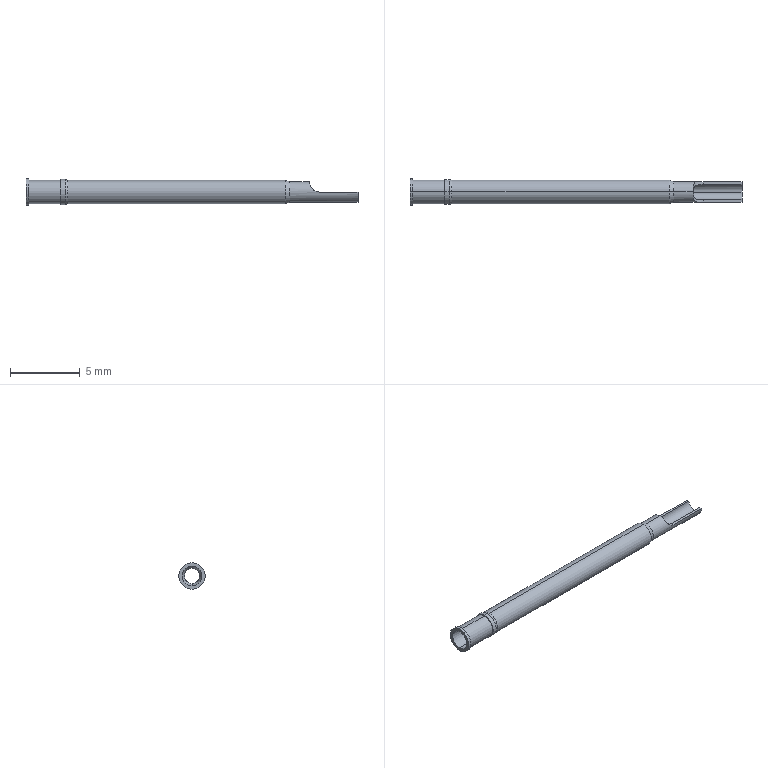Part | STEP file | Receptacle_NRB604 | 1 solid | 27 faces | box 23.8 x 1.9 x 1.9 mm | volume 15.467 mm3 | cylinder 15 | cone 6 | plane 6 | commonest cylinder face diameters 1.68 x4 1.47 x3 1.1 x2 1.4 x2 1.8 x2 1.9 x2
STEP:
#1=CARTESIAN_POINT('',(23.8,0.,-0.55));
#2=VERTEX_POINT('',#1);
#3=CARTESIAN_POINT('',(23.8,-0.55,0.));
#4=VERTEX_POINT('',#3);
#5=CARTESIAN_POINT('',(23.8,0.,0.));
#6=DIRECTION('',(-1.,0.,0.));
#7=DIRECTION('',(0.,0.,1.));
#8=AXIS2_PLACEMENT_3D('',#5,#6,#7);
#9=CIRCLE('',#8,0.55);
#10=EDGE_CURVE('',#2,#4,#9,.T.);
#11=ORIENTED_EDGE('',*,*,#10,.F.);
#12=CARTESIAN_POINT('',(18.901,0.,-0.55));
#13=VERTEX_POINT('',#12);
#14=CARTESIAN_POINT('',(23.8,0.,-0.55));
#15=DIRECTION('',(-1.,0.,0.));
#16=VECTOR('',#15,1000.);
#17=LINE('',#14,#16);
#18=EDGE_CURVE('',#2,#13,#17,.T.);
#19=ORIENTED_EDGE('',*,*,#18,.T.);
#20=CARTESIAN_POINT('',(18.901,0.,0.55));
#21=VERTEX_POINT('',#20);
#22=CARTESIAN_POINT('',(18.901,0.,0.));
#23=DIRECTION('',(-1.,0.,0.));
#24=DIRECTION('',(0.,0.,1.));
#25=AXIS2_PLACEMENT_3D('',#22,#23,#24);
#26=CIRCLE('',#25,0.55);
#27=EDGE_CURVE('',#13,#21,#26,.T.);
#28=ORIENTED_EDGE('',*,*,#27,.T.);
#29=CARTESIAN_POINT('',(20.324,0.,0.55));
#30=VERTEX_POINT('',#29);
#31=CARTESIAN_POINT('',(23.8,0.,0.55));
#32=DIRECTION('',(-1.,0.,0.));
#33=VECTOR('',#32,1000.);
#34=LINE('',#31,#33);
#35=EDGE_CURVE('',#30,#21,#34,.T.);
#36=ORIENTED_EDGE('',*,*,#35,.F.);
#37=CARTESIAN_POINT('',(21.035,-0.55,0.));
#38=VERTEX_POINT('',#37);
#39=CARTESIAN_POINT('',(21.035,-0.55,0.));
#40=CARTESIAN_POINT('',(20.928,-0.55,0.));
#41=CARTESIAN_POINT('',(20.825,-0.5513,0.02284));
#42=CARTESIAN_POINT('',(20.681,-0.5432,0.08883));
#43=CARTESIAN_POINT('',(20.636,-0.5387,0.1156));
#44=CARTESIAN_POINT('',(20.553,-0.5214,0.1779));
#45=CARTESIAN_POINT('',(20.515,-0.5085,0.2137));
#46=CARTESIAN_POINT('',(20.417,-0.4516,0.3248));
#47=CARTESIAN_POINT('',(20.375,-0.3857,0.4055));
#48=CARTESIAN_POINT('',(20.33,-0.2125,0.5177));
#49=CARTESIAN_POINT('',(20.324,-0.1056,0.55));
#50=CARTESIAN_POINT('',(20.324,0.,0.55));
#51=B_SPLINE_CURVE_WITH_KNOTS('',3,(#39,#40,#41,#42,#43,#44,#45,#46,#47,#48,#49,#50),.UNSPECIFIED.,.F.,.F.,(4,2,2,2,2,4),(0.,0.0003137,0.0004705,0.0006274,0.0009411,0.001255),.UNSPECIFIED.);
#52=EDGE_CURVE('',#38,#30,#51,.T.);
#53=ORIENTED_EDGE('',*,*,#52,.F.);
#54=CARTESIAN_POINT('',(23.8,-0.55,0.));
#55=DIRECTION('',(-1.,0.,0.));
#56=VECTOR('',#55,1000.);
#57=LINE('',#54,#56);
#58=EDGE_CURVE('',#4,#38,#57,.T.);
#59=ORIENTED_EDGE('',*,*,#58,.F.);
#60=EDGE_LOOP('',(#11,#19,#28,#36,#53,#59));
#61=FACE_OUTER_BOUND('',#60,.T.);
#62=CARTESIAN_POINT('',(23.8,0.,0.));
#63=DIRECTION('',(-1.,0.,0.));
#64=DIRECTION('',(0.,0.,1.));
#65=AXIS2_PLACEMENT_3D('',#62,#63,#64);
#66=CYLINDRICAL_SURFACE('',#65,0.55);
#67=ADVANCED_FACE('',(#61),#66,.F.);
#68=ORIENTED_EDGE('',*,*,#27,.F.);
#69=CARTESIAN_POINT('',(18.6,0.,-0.7));
#70=VERTEX_POINT('',#69);
#71=CARTESIAN_POINT('',(18.901,0.,-0.55));
#72=DIRECTION('',(-0.8949,0.,-0.4462));
#73=VECTOR('',#72,1000.);
#74=LINE('',#71,#73);
#75=EDGE_CURVE('',#13,#70,#74,.T.);
#76=ORIENTED_EDGE('',*,*,#75,.T.);
#77=CARTESIAN_POINT('',(18.6,0.,0.7));
#78=VERTEX_POINT('',#77);
#79=CARTESIAN_POINT('',(18.6,0.,0.));
#80=DIRECTION('',(-1.,0.,0.));
#81=DIRECTION('',(0.,0.,1.));
#82=AXIS2_PLACEMENT_3D('',#79,#80,#81);
#83=CIRCLE('',#82,0.7);
#84=EDGE_CURVE('',#70,#78,#83,.T.);
#85=ORIENTED_EDGE('',*,*,#84,.T.);
#86=CARTESIAN_POINT('',(18.901,0.,0.55));
#87=DIRECTION('',(-0.8949,0.,0.4462));
#88=VECTOR('',#87,1000.);
#89=LINE('',#86,#88);
#90=EDGE_CURVE('',#21,#78,#89,.T.);
#91=ORIENTED_EDGE('',*,*,#90,.F.);
#92=EDGE_LOOP('',(#68,#76,#85,#91));
#93=FACE_OUTER_BOUND('',#92,.T.);
#94=CARTESIAN_POINT('',(18.901,0.,0.));
#95=DIRECTION('',(-1.,0.,0.));
#96=DIRECTION('',(0.,0.,1.));
#97=AXIS2_PLACEMENT_3D('',#94,#95,#96);
#98=CONICAL_SURFACE('',#97,0.55,0.4625);
#99=ADVANCED_FACE('',(#93),#98,.F.);
#100=ORIENTED_EDGE('',*,*,#84,.F.);
#101=CARTESIAN_POINT('',(0.,0.,-0.7));
#102=VERTEX_POINT('',#101);
#103=CARTESIAN_POINT('',(23.8,0.,-0.7));
#104=DIRECTION('',(-1.,0.,0.));
#105=VECTOR('',#104,1000.);
#106=LINE('',#103,#105);
#107=EDGE_CURVE('',#70,#102,#106,.T.);
#108=ORIENTED_EDGE('',*,*,#107,.T.);
#109=CARTESIAN_POINT('',(0.,0.,0.7));
#110=VERTEX_POINT('',#109);
#111=CARTESIAN_POINT('',(0.,0.,0.));
#112=DIRECTION('',(-1.,0.,0.));
#113=DIRECTION('',(0.,0.,1.));
#114=AXIS2_PLACEMENT_3D('',#111,#112,#113);
#115=CIRCLE('',#114,0.7);
#116=EDGE_CURVE('',#102,#110,#115,.T.);
#117=ORIENTED_EDGE('',*,*,#116,.T.);
#118=CARTESIAN_POINT('',(23.8,0.,0.7));
#119=DIRECTION('',(-1.,0.,0.));
#120=VECTOR('',#119,1000.);
#121=LINE('',#118,#120);
#122=EDGE_CURVE('',#78,#110,#121,.T.);
#123=ORIENTED_EDGE('',*,*,#122,.F.);
#124=EDGE_LOOP('',(#100,#108,#117,#123));
#125=FACE_OUTER_BOUND('',#124,.T.);
#126=CARTESIAN_POINT('',(23.8,0.,0.));
#127=DIRECTION('',(-1.,0.,0.));
#128=DIRECTION('',(0.,0.,1.));
#129=AXIS2_PLACEMENT_3D('',#126,#127,#128);
#130=CYLINDRICAL_SURFACE('',#129,0.7);
#131=ADVANCED_FACE('',(#125),#130,.F.);
#132=CARTESIAN_POINT('',(23.8,0.735,0.));
#133=VERTEX_POINT('',#132);
#134=CARTESIAN_POINT('',(23.8,0.,-0.735));
#135=VERTEX_POINT('',#134);
#136=CARTESIAN_POINT('',(23.8,0.,0.));
#137=DIRECTION('',(-1.,0.,0.));
#138=DIRECTION('',(0.,0.,1.));
#139=AXIS2_PLACEMENT_3D('',#136,#137,#138);
#140=CIRCLE('',#139,0.735);
#141=EDGE_CURVE('',#133,#135,#140,.T.);
#142=ORIENTED_EDGE('',*,*,#141,.T.);
#143=CARTESIAN_POINT('',(18.9,0.,-0.735));
#144=VERTEX_POINT('',#143);
#145=CARTESIAN_POINT('',(23.8,0.,-0.735));
#146=DIRECTION('',(-1.,0.,0.));
#147=VECTOR('',#146,1000.);
#148=LINE('',#145,#147);
#149=EDGE_CURVE('',#135,#144,#148,.T.);
#150=ORIENTED_EDGE('',*,*,#149,.T.);
#151=CARTESIAN_POINT('',(18.9,0.,0.735));
#152=VERTEX_POINT('',#151);
#153=CARTESIAN_POINT('',(18.9,0.,0.));
#154=DIRECTION('',(-1.,0.,0.));
#155=DIRECTION('',(0.,0.,1.));
#156=AXIS2_PLACEMENT_3D('',#153,#154,#155);
#157=CIRCLE('',#156,0.735);
#158=EDGE_CURVE('',#152,#144,#157,.T.);
#159=ORIENTED_EDGE('',*,*,#158,.F.);
#160=CARTESIAN_POINT('',(20.3,0.,0.735));
#161=VERTEX_POINT('',#160);
#162=CARTESIAN_POINT('',(23.8,0.,0.735));
#163=DIRECTION('',(-1.,0.,0.));
#164=VECTOR('',#163,1000.);
#165=LINE('',#162,#164);
#166=EDGE_CURVE('',#161,#152,#165,.T.);
#167=ORIENTED_EDGE('',*,*,#166,.F.);
#168=CARTESIAN_POINT('',(21.035,0.735,0.));
#169=VERTEX_POINT('',#168);
#170=CARTESIAN_POINT('',(20.3,0.,0.735));
#171=CARTESIAN_POINT('',(20.3,0.1314,0.735));
#172=CARTESIAN_POINT('',(20.298,0.2613,0.6991));
#173=CARTESIAN_POINT('',(20.316,0.4842,0.5679));
#174=CARTESIAN_POINT('',(20.34,0.5775,0.4695));
#175=CARTESIAN_POINT('',(20.456,0.6946,0.2672));
#176=CARTESIAN_POINT('',(20.549,0.7186,0.1684));
#177=CARTESIAN_POINT('',(20.774,0.7372,0.03573));
#178=CARTESIAN_POINT('',(20.903,0.735,0.));
#179=CARTESIAN_POINT('',(21.035,0.735,0.));
#180=B_SPLINE_CURVE_WITH_KNOTS('',3,(#170,#171,#172,#173,#174,#175,#176,#177,#178,#179),.UNSPECIFIED.,.F.,.F.,(4,2,2,2,4),(0.001558,0.001947,0.002336,0.002725,0.003114),.UNSPECIFIED.);
#181=EDGE_CURVE('',#161,#169,#180,.T.);
#182=ORIENTED_EDGE('',*,*,#181,.T.);
#183=CARTESIAN_POINT('',(23.8,0.735,0.));
#184=DIRECTION('',(-1.,0.,0.));
#185=VECTOR('',#184,1000.);
#186=LINE('',#183,#185);
#187=EDGE_CURVE('',#133,#169,#186,.T.);
#188=ORIENTED_EDGE('',*,*,#187,.F.);
#189=EDGE_LOOP('',(#142,#150,#159,#167,#182,#188));
#190=FACE_OUTER_BOUND('',#189,.T.);
#191=CARTESIAN_POINT('',(23.8,0.,0.));
#192=DIRECTION('',(-1.,0.,0.));
#193=DIRECTION('',(0.,0.,1.));
#194=AXIS2_PLACEMENT_3D('',#191,#192,#193);
#195=CYLINDRICAL_SURFACE('',#194,0.735);
#196=ADVANCED_FACE('',(#190),#195,.T.);
#197=ORIENTED_EDGE('',*,*,#158,.T.);
#198=CARTESIAN_POINT('',(18.6,0.,-0.84));
#199=VERTEX_POINT('',#198);
#200=CARTESIAN_POINT('',(18.9,0.,-0.735));
#201=DIRECTION('',(-0.9439,0.,-0.3304));
#202=VECTOR('',#201,1000.);
#203=LINE('',#200,#202);
#204=EDGE_CURVE('',#144,#199,#203,.T.);
#205=ORIENTED_EDGE('',*,*,#204,.T.);
#206=CARTESIAN_POINT('',(18.6,0.,0.84));
#207=VERTEX_POINT('',#206);
#208=CARTESIAN_POINT('',(18.6,0.,0.));
#209=DIRECTION('',(-1.,0.,0.));
#210=DIRECTION('',(0.,0.,1.));
#211=AXIS2_PLACEMENT_3D('',#208,#209,#210);
#212=CIRCLE('',#211,0.84);
#213=EDGE_CURVE('',#207,#199,#212,.T.);
#214=ORIENTED_EDGE('',*,*,#213,.F.);
#215=CARTESIAN_POINT('',(18.9,0.,0.735));
#216=DIRECTION('',(-0.9439,0.,0.3304));
#217=VECTOR('',#216,1000.);
#218=LINE('',#215,#217);
#219=EDGE_CURVE('',#152,#207,#218,.T.);
#220=ORIENTED_EDGE('',*,*,#219,.F.);
#221=EDGE_LOOP('',(#197,#205,#214,#220));
#222=FACE_OUTER_BOUND('',#221,.T.);
#223=CARTESIAN_POINT('',(18.9,0.,0.));
#224=DIRECTION('',(-1.,0.,0.));
#225=DIRECTION('',(0.,0.,1.));
#226=AXIS2_PLACEMENT_3D('',#223,#224,#225);
#227=CONICAL_SURFACE('',#226,0.735,0.3367);
#228=ADVANCED_FACE('',(#222),#227,.T.);
#229=ORIENTED_EDGE('',*,*,#213,.T.);
#230=CARTESIAN_POINT('',(3.,0.,-0.84));
#231=VERTEX_POINT('',#230);
#232=CARTESIAN_POINT('',(23.8,0.,-0.84));
#233=DIRECTION('',(-1.,0.,0.));
#234=VECTOR('',#233,1000.);
#235=LINE('',#232,#234);
#236=EDGE_CURVE('',#199,#231,#235,.T.);
#237=ORIENTED_EDGE('',*,*,#236,.T.);
#238=CARTESIAN_POINT('',(3.,0.,0.84));
#239=VERTEX_POINT('',#238);
#240=CARTESIAN_POINT('',(3.,0.,0.));
#241=DIRECTION('',(-1.,0.,0.));
#242=DIRECTION('',(0.,0.,1.));
#243=AXIS2_PLACEMENT_3D('',#240,#241,#242);
#244=CIRCLE('',#243,0.84);
#245=EDGE_CURVE('',#239,#231,#244,.T.);
#246=ORIENTED_EDGE('',*,*,#245,.F.);
#247=CARTESIAN_POINT('',(23.8,0.,0.84));
#248=DIRECTION('',(-1.,0.,0.));
#249=VECTOR('',#248,1000.);
#250=LINE('',#247,#249);
#251=EDGE_CURVE('',#207,#239,#250,.T.);
#252=ORIENTED_EDGE('',*,*,#251,.F.);
#253=EDGE_LOOP('',(#229,#237,#246,#252));
#254=FACE_OUTER_BOUND('',#253,.T.);
#255=CARTESIAN_POINT('',(23.8,0.,0.));
#256=DIRECTION('',(-1.,0.,0.));
#257=DIRECTION('',(0.,0.,1.));
#258=AXIS2_PLACEMENT_3D('',#255,#256,#257);
#259=CYLINDRICAL_SURFACE('',#258,0.84);
#260=ADVANCED_FACE('',(#254),#259,.T.);
#261=ORIENTED_EDGE('',*,*,#245,.T.);
#262=CARTESIAN_POINT('',(2.8,0.,-0.9));
#263=VERTEX_POINT('',#262);
#264=CARTESIAN_POINT('',(3.,0.,-0.84));
#265=DIRECTION('',(-0.9578,0.,-0.2873));
#266=VECTOR('',#265,1000.);
#267=LINE('',#264,#266);
#268=EDGE_CURVE('',#231,#263,#267,.T.);
#269=ORIENTED_EDGE('',*,*,#268,.T.);
#270=CARTESIAN_POINT('',(2.8,0.,0.9));
#271=VERTEX_POINT('',#270);
#272=CARTESIAN_POINT('',(2.8,0.,0.));
#273=DIRECTION('',(-1.,0.,0.));
#274=DIRECTION('',(0.,0.,1.));
#275=AXIS2_PLACEMENT_3D('',#272,#273,#274);
#276=CIRCLE('',#275,0.9);
#277=EDGE_CURVE('',#271,#263,#276,.T.);
#278=ORIENTED_EDGE('',*,*,#277,.F.);
#279=CARTESIAN_POINT('',(3.,0.,0.84));
#280=DIRECTION('',(-0.9578,0.,0.2873));
#281=VECTOR('',#280,1000.);
#282=LINE('',#279,#281);
#283=EDGE_CURVE('',#239,#271,#282,.T.);
#284=ORIENTED_EDGE('',*,*,#283,.F.);
#285=EDGE_LOOP('',(#261,#269,#278,#284));
#286=FACE_OUTER_BOUND('',#285,.T.);
#287=CARTESIAN_POINT('',(3.,0.,0.));
#288=DIRECTION('',(-1.,0.,0.));
#289=DIRECTION('',(0.,0.,1.));
#290=AXIS2_PLACEMENT_3D('',#287,#288,#289);
#291=CONICAL_SURFACE('',#290,0.84,0.2915);
#292=ADVANCED_FACE('',(#286),#291,.T.);
#293=ORIENTED_EDGE('',*,*,#277,.T.);
#294=CARTESIAN_POINT('',(2.5,0.,-0.9));
#295=VERTEX_POINT('',#294);
#296=CARTESIAN_POINT('',(23.8,0.,-0.9));
#297=DIRECTION('',(-1.,0.,0.));
#298=VECTOR('',#297,1000.);
#299=LINE('',#296,#298);
#300=EDGE_CURVE('',#263,#295,#299,.T.);
#301=ORIENTED_EDGE('',*,*,#300,.T.);
#302=CARTESIAN_POINT('',(2.5,0.,0.9));
#303=VERTEX_POINT('',#302);
#304=CARTESIAN_POINT('',(2.5,0.,0.));
#305=DIRECTION('',(-1.,0.,0.));
#306=DIRECTION('',(0.,0.,1.));
#307=AXIS2_PLACEMENT_3D('',#304,#305,#306);
#308=CIRCLE('',#307,0.9);
#309=EDGE_CURVE('',#303,#295,#308,.T.);
#310=ORIENTED_EDGE('',*,*,#309,.F.);
#311=CARTESIAN_POINT('',(23.8,0.,0.9));
#312=DIRECTION('',(-1.,0.,0.));
#313=VECTOR('',#312,1000.);
#314=LINE('',#311,#313);
#315=EDGE_CURVE('',#271,#303,#314,.T.);
#316=ORIENTED_EDGE('',*,*,#315,.F.);
#317=EDGE_LOOP('',(#293,#301,#310,#316));
#318=FACE_OUTER_BOUND('',#317,.T.);
#319=CARTESIAN_POINT('',(23.8,0.,0.));
#320=DIRECTION('',(-1.,0.,0.));
#321=DIRECTION('',(0.,0.,1.));
#322=AXIS2_PLACEMENT_3D('',#319,#320,#321);
#323=CYLINDRICAL_SURFACE('',#322,0.9);
#324=ADVANCED_FACE('',(#318),#323,.T.);
#325=CARTESIAN_POINT('',(2.5,0.,0.84));
#326=VERTEX_POINT('',#325);
#327=CARTESIAN_POINT('',(2.5,0.,-0.84));
#328=VERTEX_POINT('',#327);
#329=CARTESIAN_POINT('',(2.5,0.,0.));
#330=DIRECTION('',(-1.,0.,0.));
#331=DIRECTION('',(0.,0.,1.));
#332=AXIS2_PLACEMENT_3D('',#329,#330,#331);
#333=CIRCLE('',#332,0.84);
#334=EDGE_CURVE('',#326,#328,#333,.T.);
#335=ORIENTED_EDGE('',*,*,#334,.T.);
#336=CARTESIAN_POINT('',(0.2,0.,-0.84));
#337=VERTEX_POINT('',#336);
#338=CARTESIAN_POINT('',(23.8,0.,-0.84));
#339=DIRECTION('',(-1.,0.,0.));
#340=VECTOR('',#339,1000.);
#341=LINE('',#338,#340);
#342=EDGE_CURVE('',#328,#337,#341,.T.);
#343=ORIENTED_EDGE('',*,*,#342,.T.);
#344=CARTESIAN_POINT('',(0.2,0.,0.84));
#345=VERTEX_POINT('',#344);
#346=CARTESIAN_POINT('',(0.2,0.,0.));
#347=DIRECTION('',(-1.,0.,0.));
#348=DIRECTION('',(0.,0.,1.));
#349=AXIS2_PLACEMENT_3D('',#346,#347,#348);
#350=CIRCLE('',#349,0.84);
#351=EDGE_CURVE('',#345,#337,#350,.T.);
#352=ORIENTED_EDGE('',*,*,#351,.F.);
#353=CARTESIAN_POINT('',(23.8,0.,0.84));
#354=DIRECTION('',(-1.,0.,0.));
#355=VECTOR('',#354,1000.);
#356=LINE('',#353,#355);
#357=EDGE_CURVE('',#326,#345,#356,.T.);
#358=ORIENTED_EDGE('',*,*,#357,.F.);
#359=EDGE_LOOP('',(#335,#343,#352,#358));
#360=FACE_OUTER_BOUND('',#359,.T.);
#361=CARTESIAN_POINT('',(23.8,0.,0.));
#362=DIRECTION('',(-1.,0.,0.));
#363=DIRECTION('',(0.,0.,1.));
#364=AXIS2_PLACEMENT_3D('',#361,#362,#363);
#365=CYLINDRICAL_SURFACE('',#364,0.84);
#366=ADVANCED_FACE('',(#360),#365,.T.);
#367=CARTESIAN_POINT('',(0.2,0.,0.95));
#368=VERTEX_POINT('',#367);
#369=CARTESIAN_POINT('',(0.2,0.,-0.95));
#370=VERTEX_POINT('',#369);
#371=CARTESIAN_POINT('',(0.2,0.,0.));
#372=DIRECTION('',(-1.,0.,0.));
#373=DIRECTION('',(0.,0.,1.));
#374=AXIS2_PLACEMENT_3D('',#371,#372,#373);
#375=CIRCLE('',#374,0.95);
#376=EDGE_CURVE('',#368,#370,#375,.T.);
#377=ORIENTED_EDGE('',*,*,#376,.T.);
#378=CARTESIAN_POINT('',(0.,0.,-0.95));
#379=VERTEX_POINT('',#378);
#380=CARTESIAN_POINT('',(23.8,0.,-0.95));
#381=DIRECTION('',(-1.,0.,0.));
#382=VECTOR('',#381,1000.);
#383=LINE('',#380,#382);
#384=EDGE_CURVE('',#370,#379,#383,.T.);
#385=ORIENTED_EDGE('',*,*,#384,.T.);
#386=CARTESIAN_POINT('',(0.,0.,0.95));
#387=VERTEX_POINT('',#386);
#388=CARTESIAN_POINT('',(0.,0.,0.));
#389=DIRECTION('',(-1.,0.,0.));
#390=DIRECTION('',(0.,0.,1.));
#391=AXIS2_PLACEMENT_3D('',#388,#389,#390);
#392=CIRCLE('',#391,0.95);
#393=EDGE_CURVE('',#387,#379,#392,.T.);
#394=ORIENTED_EDGE('',*,*,#393,.F.);
#395=CARTESIAN_POINT('',(23.8,0.,0.95));
#396=DIRECTION('',(-1.,0.,0.));
#397=VECTOR('',#396,1000.);
#398=LINE('',#395,#397);
#399=EDGE_CURVE('',#368,#387,#398,.T.);
#400=ORIENTED_EDGE('',*,*,#399,.F.);
#401=EDGE_LOOP('',(#377,#385,#394,#400));
#402=FACE_OUTER_BOUND('',#401,.T.);
#403=CARTESIAN_POINT('',(23.8,0.,0.));
#404=DIRECTION('',(-1.,0.,0.));
#405=DIRECTION('',(0.,0.,1.));
#406=AXIS2_PLACEMENT_3D('',#403,#404,#405);
#407=CYLINDRICAL_SURFACE('',#406,0.95);
#408=ADVANCED_FACE('',(#402),#407,.T.);
#409=ORIENTED_EDGE('',*,*,#393,.T.);
#410=CARTESIAN_POINT('',(0.,0.,0.));
#411=DIRECTION('',(-1.,0.,0.));
#412=DIRECTION('',(0.,0.,1.));
#413=AXIS2_PLACEMENT_3D('',#410,#411,#412);
#414=CIRCLE('',#413,0.95);
#415=EDGE_CURVE('',#379,#387,#414,.T.);
#416=ORIENTED_EDGE('',*,*,#415,.T.);
#417=EDGE_LOOP('',(#409,#416));
#418=FACE_OUTER_BOUND('',#417,.T.);
#419=CARTESIAN_POINT('',(0.,0.,0.));
#420=DIRECTION('',(-1.,0.,0.));
#421=DIRECTION('',(0.,0.,1.));
#422=AXIS2_PLACEMENT_3D('',#419,#420,#421);
#423=CIRCLE('',#422,0.7);
#424=EDGE_CURVE('',#110,#102,#423,.T.);
#425=ORIENTED_EDGE('',*,*,#424,.F.);
#426=ORIENTED_EDGE('',*,*,#116,.F.);
#427=EDGE_LOOP('',(#425,#426));
#428=FACE_BOUND('',#427,.T.);
#429=CARTESIAN_POINT('',(0.,0.,0.));
#430=DIRECTION('',(1.,0.,0.));
#431=DIRECTION('',(0.,0.,-1.));
#432=AXIS2_PLACEMENT_3D('',#429,#430,#431);
#433=PLANE('',#432);
#434=ADVANCED_FACE('',(#418,#428),#433,.F.);
#435=ORIENTED_EDGE('',*,*,#141,.F.);
#436=CARTESIAN_POINT('',(23.8,0.55,0.));
#437=VERTEX_POINT('',#436);
#438=CARTESIAN_POINT('',(23.8,-0.735,0.));
#439=DIRECTION('',(0.,1.,0.));
#440=VECTOR('',#439,1000.);
#441=LINE('',#438,#440);
#442=EDGE_CURVE('',#437,#133,#441,.T.);
#443=ORIENTED_EDGE('',*,*,#442,.F.);
#444=CARTESIAN_POINT('',(23.8,0.,0.));
#445=DIRECTION('',(-1.,0.,0.));
#446=DIRECTION('',(0.,0.,1.));
#447=AXIS2_PLACEMENT_3D('',#444,#445,#446);
#448=CIRCLE('',#447,0.55);
#449=EDGE_CURVE('',#437,#2,#448,.T.);
#450=ORIENTED_EDGE('',*,*,#449,.T.);
#451=ORIENTED_EDGE('',*,*,#10,.T.);
#452=CARTESIAN_POINT('',(23.8,-0.735,0.));
#453=VERTEX_POINT('',#452);
#454=CARTESIAN_POINT('',(23.8,-0.735,0.));
#455=DIRECTION('',(0.,1.,0.));
#456=VECTOR('',#455,1000.);
#457=LINE('',#454,#456);
#458=EDGE_CURVE('',#453,#4,#457,.T.);
#459=ORIENTED_EDGE('',*,*,#458,.F.);
#460=CARTESIAN_POINT('',(23.8,0.,0.));
#461=DIRECTION('',(-1.,0.,0.));
#462=DIRECTION('',(0.,0.,1.));
#463=AXIS2_PLACEMENT_3D('',#460,#461,#462);
#464=CIRCLE('',#463,0.735);
#465=EDGE_CURVE('',#135,#453,#464,.T.);
#466=ORIENTED_EDGE('',*,*,#465,.F.);
#467=EDGE_LOOP('',(#435,#443,#450,#451,#459,#466));
#468=FACE_OUTER_BOUND('',#467,.T.);
#469=CARTESIAN_POINT('',(23.8,0.735,0.));
#470=DIRECTION('',(-1.,0.,0.));
#471=DIRECTION('',(0.,0.,1.));
#472=AXIS2_PLACEMENT_3D('',#469,#470,#471);
#473=PLANE('',#472);
#474=ADVANCED_FACE('',(#468),#473,.F.);
#475=ORIENTED_EDGE('',*,*,#384,.F.);
#476=CARTESIAN_POINT('',(0.2,0.,0.));
#477=DIRECTION('',(-1.,0.,0.));
#478=DIRECTION('',(0.,0.,1.));
#479=AXIS2_PLACEMENT_3D('',#476,#477,#478);
#480=CIRCLE('',#479,0.95);
#481=EDGE_CURVE('',#370,#368,#480,.T.);
#482=ORIENTED_EDGE('',*,*,#481,.T.);
#483=ORIENTED_EDGE('',*,*,#399,.T.);
#484=ORIENTED_EDGE('',*,*,#415,.F.);
#485=EDGE_LOOP('',(#475,#482,#483,#484));
#486=FACE_OUTER_BOUND('',#485,.T.);
#487=CARTESIAN_POINT('',(23.8,0.,0.));
#488=DIRECTION('',(-1.,0.,0.));
#489=DIRECTION('',(0.,0.,1.));
#490=AXIS2_PLACEMENT_3D('',#487,#488,#489);
#491=CYLINDRICAL_SURFACE('',#490,0.95);
#492=ADVANCED_FACE('',(#486),#491,.T.);
#493=ORIENTED_EDGE('',*,*,#376,.F.);
#494=ORIENTED_EDGE('',*,*,#481,.F.);
#495=EDGE_LOOP('',(#493,#494));
#496=FACE_OUTER_BOUND('',#495,.T.);
#497=ORIENTED_EDGE('',*,*,#351,.T.);
#498=CARTESIAN_POINT('',(0.2,0.,0.));
#499=DIRECTION('',(-1.,0.,0.));
#500=DIRECTION('',(0.,0.,1.));
#501=AXIS2_PLACEMENT_3D('',#498,#499,#500);
#502=CIRCLE('',#501,0.84);
#503=EDGE_CURVE('',#337,#345,#502,.T.);
#504=ORIENTED_EDGE('',*,*,#503,.T.);
#505=EDGE_LOOP('',(#497,#504));
#506=FACE_BOUND('',#505,.T.);
#507=CARTESIAN_POINT('',(0.2,0.95,0.));
#508=DIRECTION('',(-1.,0.,0.));
#509=DIRECTION('',(0.,0.,1.));
#510=AXIS2_PLACEMENT_3D('',#507,#508,#509);
#511=PLANE('',#510);
#512=ADVANCED_FACE('',(#496,#506),#511,.F.);
#513=ORIENTED_EDGE('',*,*,#342,.F.);
#514=CARTESIAN_POINT('',(2.5,0.,0.));
#515=DIRECTION('',(-1.,0.,0.));
#516=DIRECTION('',(0.,0.,1.));
#517=AXIS2_PLACEMENT_3D('',#514,#515,#516);
#518=CIRCLE('',#517,0.84);
#519=EDGE_CURVE('',#328,#326,#518,.T.);
#520=ORIENTED_EDGE('',*,*,#519,.T.);
#521=ORIENTED_EDGE('',*,*,#357,.T.);
#522=ORIENTED_EDGE('',*,*,#503,.F.);
#523=EDGE_LOOP('',(#513,#520,#521,#522));
#524=FACE_OUTER_BOUND('',#523,.T.);
#525=CARTESIAN_POINT('',(23.8,0.,0.));
#526=DIRECTION('',(-1.,0.,0.));
#527=DIRECTION('',(0.,0.,1.));
#528=AXIS2_PLACEMENT_3D('',#525,#526,#527);
#529=CYLINDRICAL_SURFACE('',#528,0.84);
#530=ADVANCED_FACE('',(#524),#529,.T.);
#531=ORIENTED_EDGE('',*,*,#334,.F.);
#532=ORIENTED_EDGE('',*,*,#519,.F.);
#533=EDGE_LOOP('',(#531,#532));
#534=FACE_BOUND('',#533,.T.);
#535=ORIENTED_EDGE('',*,*,#309,.T.);
#536=CARTESIAN_POINT('',(2.5,0.,0.));
#537=DIRECTION('',(-1.,0.,0.));
#538=DIRECTION('',(0.,0.,1.));
#539=AXIS2_PLACEMENT_3D('',#536,#537,#538);
#540=CIRCLE('',#539,0.9);
#541=EDGE_CURVE('',#295,#303,#540,.T.);
#542=ORIENTED_EDGE('',*,*,#541,.T.);
#543=EDGE_LOOP('',(#535,#542));
#544=FACE_OUTER_BOUND('',#543,.T.);
#545=CARTESIAN_POINT('',(2.5,0.84,0.));
#546=DIRECTION('',(1.,0.,0.));
#547=DIRECTION('',(0.,0.,-1.));
#548=AXIS2_PLACEMENT_3D('',#545,#546,#547);
#549=PLANE('',#548);
#550=ADVANCED_FACE('',(#534,#544),#549,.F.);
#551=ORIENTED_EDGE('',*,*,#300,.F.);
#552=CARTESIAN_POINT('',(2.8,0.,0.));
#553=DIRECTION('',(-1.,0.,0.));
#554=DIRECTION('',(0.,0.,1.));
#555=AXIS2_PLACEMENT_3D('',#552,#553,#554);
#556=CIRCLE('',#555,0.9);
#557=EDGE_CURVE('',#263,#271,#556,.T.);
#558=ORIENTED_EDGE('',*,*,#557,.T.);
#559=ORIENTED_EDGE('',*,*,#315,.T.);
#560=ORIENTED_EDGE('',*,*,#541,.F.);
#561=EDGE_LOOP('',(#551,#558,#559,#560));
#562=FACE_OUTER_BOUND('',#561,.T.);
#563=CARTESIAN_POINT('',(23.8,0.,0.));
#564=DIRECTION('',(-1.,0.,0.));
#565=DIRECTION('',(0.,0.,1.));
#566=AXIS2_PLACEMENT_3D('',#563,#564,#565);
#567=CYLINDRICAL_SURFACE('',#566,0.9);
#568=ADVANCED_FACE('',(#562),#567,.T.);
#569=ORIENTED_EDGE('',*,*,#268,.F.);
#570=CARTESIAN_POINT('',(3.,0.,0.));
#571=DIRECTION('',(-1.,0.,0.));
#572=DIRECTION('',(0.,0.,1.));
#573=AXIS2_PLACEMENT_3D('',#570,#571,#572);
#574=CIRCLE('',#573,0.84);
#575=EDGE_CURVE('',#231,#239,#574,.T.);
#576=ORIENTED_EDGE('',*,*,#575,.T.);
#577=ORIENTED_EDGE('',*,*,#283,.T.);
#578=ORIENTED_EDGE('',*,*,#557,.F.);
#579=EDGE_LOOP('',(#569,#576,#577,#578));
#580=FACE_OUTER_BOUND('',#579,.T.);
#581=CARTESIAN_POINT('',(3.,0.,0.));
#582=DIRECTION('',(-1.,0.,0.));
#583=DIRECTION('',(0.,0.,1.));
#584=AXIS2_PLACEMENT_3D('',#581,#582,#583);
#585=CONICAL_SURFACE('',#584,0.84,0.2915);
#586=ADVANCED_FACE('',(#580),#585,.T.);
#587=ORIENTED_EDGE('',*,*,#236,.F.);
#588=CARTESIAN_POINT('',(18.6,0.,0.));
#589=DIRECTION('',(-1.,0.,0.));
#590=DIRECTION('',(0.,0.,1.));
#591=AXIS2_PLACEMENT_3D('',#588,#589,#590);
#592=CIRCLE('',#591,0.84);
#593=EDGE_CURVE('',#199,#207,#592,.T.);
#594=ORIENTED_EDGE('',*,*,#593,.T.);
#595=ORIENTED_EDGE('',*,*,#251,.T.);
#596=ORIENTED_EDGE('',*,*,#575,.F.);
#597=EDGE_LOOP('',(#587,#594,#595,#596));
#598=FACE_OUTER_BOUND('',#597,.T.);
#599=CARTESIAN_POINT('',(23.8,0.,0.));
#600=DIRECTION('',(-1.,0.,0.));
#601=DIRECTION('',(0.,0.,1.));
#602=AXIS2_PLACEMENT_3D('',#599,#600,#601);
#603=CYLINDRICAL_SURFACE('',#602,0.84);
#604=ADVANCED_FACE('',(#598),#603,.T.);
#605=ORIENTED_EDGE('',*,*,#204,.F.);
#606=CARTESIAN_POINT('',(18.9,0.,0.));
#607=DIRECTION('',(-1.,0.,0.));
#608=DIRECTION('',(0.,0.,1.));
#609=AXIS2_PLACEMENT_3D('',#606,#607,#608);
#610=CIRCLE('',#609,0.735);
#611=EDGE_CURVE('',#144,#152,#610,.T.);
#612=ORIENTED_EDGE('',*,*,#611,.T.);
#613=ORIENTED_EDGE('',*,*,#219,.T.);
#614=ORIENTED_EDGE('',*,*,#593,.F.);
#615=EDGE_LOOP('',(#605,#612,#613,#614));
#616=FACE_OUTER_BOUND('',#615,.T.);
#617=CARTESIAN_POINT('',(18.9,0.,0.));
#618=DIRECTION('',(-1.,0.,0.));
#619=DIRECTION('',(0.,0.,1.));
#620=AXIS2_PLACEMENT_3D('',#617,#618,#619);
#621=CONICAL_SURFACE('',#620,0.735,0.3367);
#622=ADVANCED_FACE('',(#616),#621,.T.);
#623=ORIENTED_EDGE('',*,*,#149,.F.);
#624=ORIENTED_EDGE('',*,*,#465,.T.);
#625=CARTESIAN_POINT('',(21.035,-0.735,0.));
#626=VERTEX_POINT('',#625);
#627=CARTESIAN_POINT('',(23.8,-0.735,0.));
#628=DIRECTION('',(-1.,0.,0.));
#629=VECTOR('',#628,1000.);
#630=LINE('',#627,#629);
#631=EDGE_CURVE('',#453,#626,#630,.T.);
#632=ORIENTED_EDGE('',*,*,#631,.T.);
#633=CARTESIAN_POINT('',(21.035,-0.735,0.));
#634=CARTESIAN_POINT('',(20.903,-0.735,0.));
#635=CARTESIAN_POINT('',(20.774,-0.7371,0.0359));
#636=CARTESIAN_POINT('',(20.551,-0.7188,0.1672));
#637=CARTESIAN_POINT('',(20.457,-0.6951,0.2658));
#638=CARTESIAN_POINT('',(20.34,-0.5788,0.4678));
#639=CARTESIAN_POINT('',(20.316,-0.4858,0.5668));
#640=CARTESIAN_POINT('',(20.298,-0.2612,0.6993));
#641=CARTESIAN_POINT('',(20.3,-0.1316,0.735));
#642=CARTESIAN_POINT('',(20.3,0.,0.735));
#643=B_SPLINE_CURVE_WITH_KNOTS('',3,(#633,#634,#635,#636,#637,#638,#639,#640,#641,#642),.UNSPECIFIED.,.F.,.F.,(4,2,2,2,4),(0.,0.0003894,0.0007789,0.001168,0.001558),.UNSPECIFIED.);
#644=EDGE_CURVE('',#626,#161,#643,.T.);
#645=ORIENTED_EDGE('',*,*,#644,.T.);
#646=ORIENTED_EDGE('',*,*,#166,.T.);
#647=ORIENTED_EDGE('',*,*,#611,.F.);
#648=EDGE_LOOP('',(#623,#624,#632,#645,#646,#647));
#649=FACE_OUTER_BOUND('',#648,.T.);
#650=CARTESIAN_POINT('',(23.8,0.,0.));
#651=DIRECTION('',(-1.,0.,0.));
#652=DIRECTION('',(0.,0.,1.));
#653=AXIS2_PLACEMENT_3D('',#650,#651,#652);
#654=CYLINDRICAL_SURFACE('',#653,0.735);
#655=ADVANCED_FACE('',(#649),#654,.T.);
#656=ORIENTED_EDGE('',*,*,#107,.F.);
#657=CARTESIAN_POINT('',(18.6,0.,0.));
#658=DIRECTION('',(-1.,0.,0.));
#659=DIRECTION('',(0.,0.,1.));
#660=AXIS2_PLACEMENT_3D('',#657,#658,#659);
#661=CIRCLE('',#660,0.7);
#662=EDGE_CURVE('',#78,#70,#661,.T.);
#663=ORIENTED_EDGE('',*,*,#662,.F.);
#664=ORIENTED_EDGE('',*,*,#122,.T.);
#665=ORIENTED_EDGE('',*,*,#424,.T.);
#666=EDGE_LOOP('',(#656,#663,#664,#665));
#667=FACE_OUTER_BOUND('',#666,.T.);
#668=CARTESIAN_POINT('',(23.8,0.,0.));
#669=DIRECTION('',(-1.,0.,0.));
#670=DIRECTION('',(0.,0.,1.));
#671=AXIS2_PLACEMENT_3D('',#668,#669,#670);
#672=CYLINDRICAL_SURFACE('',#671,0.7);
#673=ADVANCED_FACE('',(#667),#672,.F.);
#674=ORIENTED_EDGE('',*,*,#75,.F.);
#675=CARTESIAN_POINT('',(18.901,0.,0.));
#676=DIRECTION('',(-1.,0.,0.));
#677=DIRECTION('',(0.,0.,1.));
#678=AXIS2_PLACEMENT_3D('',#675,#676,#677);
#679=CIRCLE('',#678,0.55);
#680=EDGE_CURVE('',#21,#13,#679,.T.);
#681=ORIENTED_EDGE('',*,*,#680,.F.);
#682=ORIENTED_EDGE('',*,*,#90,.T.);
#683=ORIENTED_EDGE('',*,*,#662,.T.);
#684=EDGE_LOOP('',(#674,#681,#682,#683));
#685=FACE_OUTER_BOUND('',#684,.T.);
#686=CARTESIAN_POINT('',(18.901,0.,0.));
#687=DIRECTION('',(-1.,0.,0.));
#688=DIRECTION('',(0.,0.,1.));
#689=AXIS2_PLACEMENT_3D('',#686,#687,#688);
#690=CONICAL_SURFACE('',#689,0.55,0.4625);
#691=ADVANCED_FACE('',(#685),#690,.F.);
#692=ORIENTED_EDGE('',*,*,#18,.F.);
#693=ORIENTED_EDGE('',*,*,#449,.F.);
#694=CARTESIAN_POINT('',(21.035,0.55,0.));
#695=VERTEX_POINT('',#694);
#696=CARTESIAN_POINT('',(23.8,0.55,0.));
#697=DIRECTION('',(1.,0.,0.));
#698=VECTOR('',#697,1000.);
#699=LINE('',#696,#698);
#700=EDGE_CURVE('',#695,#437,#699,.T.);
#701=ORIENTED_EDGE('',*,*,#700,.F.);
#702=CARTESIAN_POINT('',(20.324,0.,0.55));
#703=CARTESIAN_POINT('',(20.324,0.1053,0.55));
#704=CARTESIAN_POINT('',(20.33,0.211,0.5183));
#705=CARTESIAN_POINT('',(20.375,0.385,0.4062));
#706=CARTESIAN_POINT('',(20.415,0.45,0.3273));
#707=CARTESIAN_POINT('',(20.546,0.5274,0.1775));
#708=CARTESIAN_POINT('',(20.631,0.5404,0.1117));
#709=CARTESIAN_POINT('',(20.824,0.5513,0.02318));
#710=CARTESIAN_POINT('',(20.929,0.55,0.));
#711=CARTESIAN_POINT('',(21.035,0.55,0.));
#712=B_SPLINE_CURVE_WITH_KNOTS('',3,(#702,#703,#704,#705,#706,#707,#708,#709,#710,#711),.UNSPECIFIED.,.F.,.F.,(4,2,2,2,4),(0.001255,0.001568,0.00188,0.002193,0.002506),.UNSPECIFIED.);
#713=EDGE_CURVE('',#30,#695,#712,.T.);
#714=ORIENTED_EDGE('',*,*,#713,.F.);
#715=ORIENTED_EDGE('',*,*,#35,.T.);
#716=ORIENTED_EDGE('',*,*,#680,.T.);
#717=EDGE_LOOP('',(#692,#693,#701,#714,#715,#716));
#718=FACE_OUTER_BOUND('',#717,.T.);
#719=CARTESIAN_POINT('',(23.8,0.,0.));
#720=DIRECTION('',(-1.,0.,0.));
#721=DIRECTION('',(0.,0.,1.));
#722=AXIS2_PLACEMENT_3D('',#719,#720,#721);
#723=CYLINDRICAL_SURFACE('',#722,0.55);
#724=ADVANCED_FACE('',(#718),#723,.F.);
#725=CARTESIAN_POINT('',(21.035,-0.735,0.));
#726=DIRECTION('',(0.,1.,0.));
#727=VECTOR('',#726,1000.);
#728=LINE('',#725,#727);
#729=EDGE_CURVE('',#626,#38,#728,.T.);
#730=ORIENTED_EDGE('',*,*,#729,.T.);
#731=ORIENTED_EDGE('',*,*,#52,.T.);
#732=ORIENTED_EDGE('',*,*,#713,.T.);
#733=CARTESIAN_POINT('',(21.035,-0.735,0.));
#734=DIRECTION('',(0.,1.,0.));
#735=VECTOR('',#734,1000.);
#736=LINE('',#733,#735);
#737=EDGE_CURVE('',#695,#169,#736,.T.);
#738=ORIENTED_EDGE('',*,*,#737,.T.);
#739=ORIENTED_EDGE('',*,*,#181,.F.);
#740=ORIENTED_EDGE('',*,*,#644,.F.);
#741=EDGE_LOOP('',(#730,#731,#732,#738,#739,#740));
#742=FACE_OUTER_BOUND('',#741,.T.);
#743=CARTESIAN_POINT('',(21.035,-0.735,0.735));
#744=DIRECTION('',(0.,1.,0.));
#745=DIRECTION('',(0.,0.,1.));
#746=AXIS2_PLACEMENT_3D('',#743,#744,#745);
#747=CYLINDRICAL_SURFACE('',#746,0.735);
#748=ADVANCED_FACE('',(#742),#747,.F.);
#749=ORIENTED_EDGE('',*,*,#58,.T.);
#750=ORIENTED_EDGE('',*,*,#729,.F.);
#751=ORIENTED_EDGE('',*,*,#631,.F.);
#752=ORIENTED_EDGE('',*,*,#458,.T.);
#753=EDGE_LOOP('',(#749,#750,#751,#752));
#754=FACE_OUTER_BOUND('',#753,.T.);
#755=CARTESIAN_POINT('',(23.8,-0.735,0.));
#756=DIRECTION('',(0.,0.,-1.));
#757=DIRECTION('',(-1.,0.,0.));
#758=AXIS2_PLACEMENT_3D('',#755,#756,#757);
#759=PLANE('',#758);
#760=ADVANCED_FACE('',(#754),#759,.F.);
#761=ORIENTED_EDGE('',*,*,#700,.T.);
#762=ORIENTED_EDGE('',*,*,#442,.T.);
#763=ORIENTED_EDGE('',*,*,#187,.T.);
#764=ORIENTED_EDGE('',*,*,#737,.F.);
#765=EDGE_LOOP('',(#761,#762,#763,#764));
#766=FACE_OUTER_BOUND('',#765,.T.);
#767=CARTESIAN_POINT('',(23.8,-0.735,0.));
#768=DIRECTION('',(0.,0.,-1.));
#769=DIRECTION('',(-1.,0.,0.));
#770=AXIS2_PLACEMENT_3D('',#767,#768,#769);
#771=PLANE('',#770);
#772=ADVANCED_FACE('',(#766),#771,.F.);
#773=CLOSED_SHELL('',(#67,#99,#131,#196,#228,#260,#292,#324,#366,#408,#434,#474,#492,#512,#530,#550,#568,#586,#604,#622,#655,#673,#691,#724,#748,#760,#772));
#774=MANIFOLD_SOLID_BREP('',#773);
#775=CARTESIAN_POINT('',(0.,0.,0.));
#776=DIRECTION('',(0.,0.,1.));
#777=DIRECTION('',(1.,0.,0.));
#778=AXIS2_PLACEMENT_3D('',#775,#776,#777);
#779=(LENGTH_UNIT()NAMED_UNIT(*)SI_UNIT(.MILLI.,.METRE.));
#780=UNCERTAINTY_MEASURE_WITH_UNIT(LENGTH_MEASURE(0.00001),#779,'','');
#781=(NAMED_UNIT(*)PLANE_ANGLE_UNIT()SI_UNIT($,.RADIAN.));
#782=(NAMED_UNIT(*)SI_UNIT($,.STERADIAN.)SOLID_ANGLE_UNIT());
#783=(GEOMETRIC_REPRESENTATION_CONTEXT(3)GLOBAL_UNCERTAINTY_ASSIGNED_CONTEXT((#780))GLOBAL_UNIT_ASSIGNED_CONTEXT((#779,#781,#782))REPRESENTATION_CONTEXT('',''));
#784=ADVANCED_BREP_SHAPE_REPRESENTATION('',(#774,#778),#783);